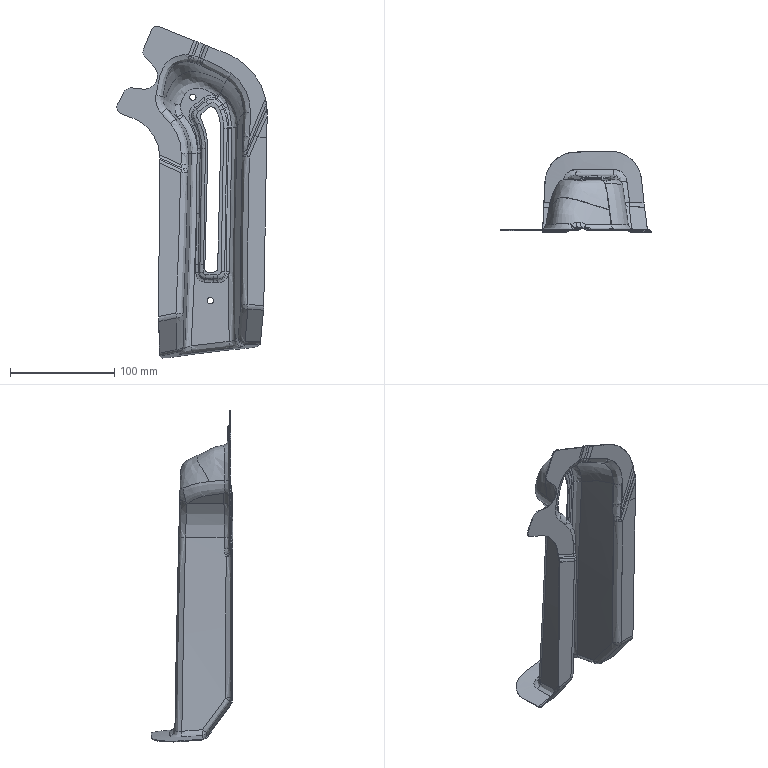Part | STEP file | FNA5401852 | 1 solid | 315 faces | box 144.073 x 78.491 x 318.118 mm | volume 43750 mm3 | spline 252 | plane 22 | cylinder 19 | other 18 | sphere 4 | commonest cylinder face diameters 8 x4 6.4 x2 9.6 x2 12 x2 12.4 x2 14 x2